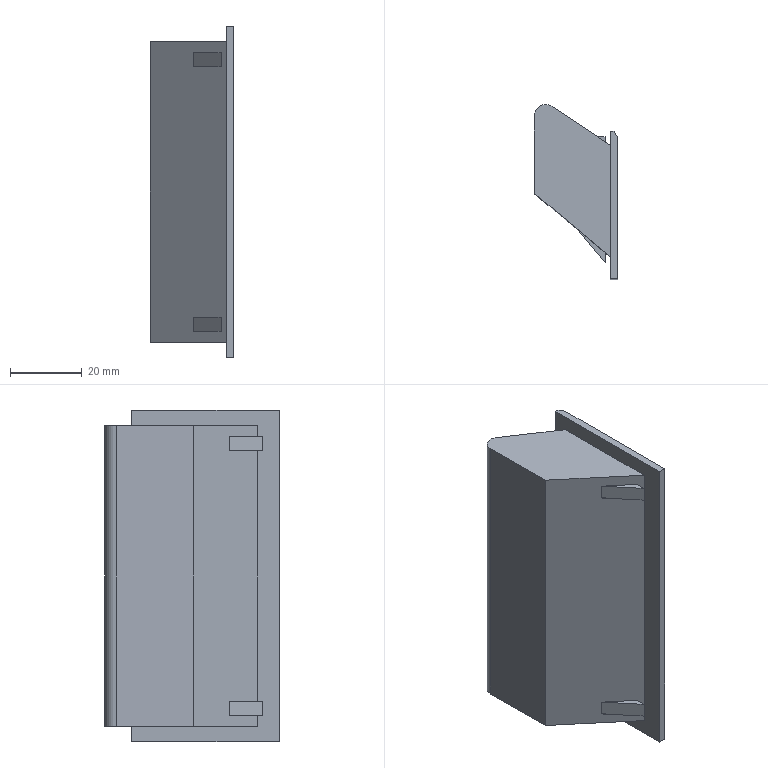Part | SolidWorks | features BaseBody 1 | 1 solid | 54 faces | box 23.155 x 48.5 x 92 mm | volume 9910 mm3 | plane 52 | cylinder 2 | commonest cylinder face diameters 4 x1 6.309 x1
STEP:
#1=CARTESIAN_POINT('',(-22.,24.19,40.75));
#2=VERTEX_POINT('',#1);
#3=CARTESIAN_POINT('',(0.,5.73,40.75));
#4=VERTEX_POINT('',#3);
#5=CARTESIAN_POINT('',(-22.,24.19,40.75));
#6=DIRECTION('',(0.766,-0.6428,0.));
#7=VECTOR('',#6,1000.);
#8=LINE('',#5,#7);
#9=EDGE_CURVE('',#2,#4,#8,.T.);
#10=ORIENTED_EDGE('',*,*,#9,.T.);
#11=CARTESIAN_POINT('',(0.,5.73,-40.75));
#12=VERTEX_POINT('',#11);
#13=CARTESIAN_POINT('',(0.,5.73,40.75));
#14=DIRECTION('',(0.,0.,-1.));
#15=VECTOR('',#14,1000.);
#16=LINE('',#13,#15);
#17=EDGE_CURVE('',#4,#12,#16,.T.);
#18=ORIENTED_EDGE('',*,*,#17,.T.);
#19=CARTESIAN_POINT('',(-22.,24.19,-40.75));
#20=VERTEX_POINT('',#19);
#21=CARTESIAN_POINT('',(-22.,24.19,-40.75));
#22=DIRECTION('',(-0.766,0.6428,0.));
#23=VECTOR('',#22,1000.);
#24=LINE('',#21,#23);
#25=EDGE_CURVE('',#12,#20,#24,.T.);
#26=ORIENTED_EDGE('',*,*,#25,.T.);
#27=CARTESIAN_POINT('',(-22.,24.19,40.75));
#28=DIRECTION('',(0.,0.,1.));
#29=VECTOR('',#28,1000.);
#30=LINE('',#27,#29);
#31=EDGE_CURVE('',#20,#2,#30,.T.);
#32=ORIENTED_EDGE('',*,*,#31,.T.);
#33=EDGE_LOOP('',(#10,#18,#26,#32));
#34=FACE_OUTER_BOUND('',#33,.T.);
#35=CARTESIAN_POINT('',(-22.,24.19,40.75));
#36=DIRECTION('',(0.6428,0.766,0.));
#37=DIRECTION('',(-0.766,0.6428,0.));
#38=AXIS2_PLACEMENT_3D('',#35,#36,#37);
#39=PLANE('',#38);
#40=ADVANCED_FACE('',(#34),#39,.T.);
#41=CARTESIAN_POINT('',(0.,39.268,46.));
#42=VERTEX_POINT('',#41);
#43=CARTESIAN_POINT('',(0.,39.268,-46.));
#44=VERTEX_POINT('',#43);
#45=CARTESIAN_POINT('',(0.,39.268,46.));
#46=DIRECTION('',(0.,0.,-1.));
#47=VECTOR('',#46,1000.);
#48=LINE('',#45,#47);
#49=EDGE_CURVE('',#42,#44,#48,.T.);
#50=ORIENTED_EDGE('',*,*,#49,.F.);
#51=CARTESIAN_POINT('',(0.,0.,46.));
#52=VERTEX_POINT('',#51);
#53=CARTESIAN_POINT('',(0.,0.,46.));
#54=DIRECTION('',(0.,1.,0.));
#55=VECTOR('',#54,1000.);
#56=LINE('',#53,#55);
#57=EDGE_CURVE('',#52,#42,#56,.T.);
#58=ORIENTED_EDGE('',*,*,#57,.F.);
#59=CARTESIAN_POINT('',(0.,0.,-46.));
#60=VERTEX_POINT('',#59);
#61=CARTESIAN_POINT('',(0.,0.,46.));
#62=DIRECTION('',(0.,0.,1.));
#63=VECTOR('',#62,1000.);
#64=LINE('',#61,#63);
#65=EDGE_CURVE('',#60,#52,#64,.T.);
#66=ORIENTED_EDGE('',*,*,#65,.F.);
#67=CARTESIAN_POINT('',(0.,0.,-46.));
#68=DIRECTION('',(0.,-1.,0.));
#69=VECTOR('',#68,1000.);
#70=LINE('',#67,#69);
#71=EDGE_CURVE('',#44,#60,#70,.T.);
#72=ORIENTED_EDGE('',*,*,#71,.F.);
#73=EDGE_LOOP('',(#50,#58,#66,#72));
#74=FACE_OUTER_BOUND('',#73,.T.);
#75=CARTESIAN_POINT('',(0.,35.072,40.75));
#76=VERTEX_POINT('',#75);
#77=CARTESIAN_POINT('',(0.,0.,40.75));
#78=DIRECTION('',(0.,-1.,0.));
#79=VECTOR('',#78,1000.);
#80=LINE('',#77,#79);
#81=EDGE_CURVE('',#76,#4,#80,.T.);
#82=ORIENTED_EDGE('',*,*,#81,.F.);
#83=CARTESIAN_POINT('',(0.,35.072,-40.75));
#84=VERTEX_POINT('',#83);
#85=CARTESIAN_POINT('',(0.,35.072,46.));
#86=DIRECTION('',(0.,0.,1.));
#87=VECTOR('',#86,1000.);
#88=LINE('',#85,#87);
#89=EDGE_CURVE('',#84,#76,#88,.T.);
#90=ORIENTED_EDGE('',*,*,#89,.F.);
#91=CARTESIAN_POINT('',(0.,0.,-40.75));
#92=DIRECTION('',(0.,1.,0.));
#93=VECTOR('',#92,1000.);
#94=LINE('',#91,#93);
#95=EDGE_CURVE('',#12,#84,#94,.T.);
#96=ORIENTED_EDGE('',*,*,#95,.F.);
#97=ORIENTED_EDGE('',*,*,#17,.F.);
#98=EDGE_LOOP('',(#82,#90,#96,#97));
#99=FACE_BOUND('',#98,.T.);
#100=CARTESIAN_POINT('',(0.,0.,46.));
#101=DIRECTION('',(-1.,0.,0.));
#102=DIRECTION('',(0.,0.,1.));
#103=AXIS2_PLACEMENT_3D('',#100,#101,#102);
#104=PLANE('',#103);
#105=ADVANCED_FACE('',(#74,#99),#104,.F.);
#106=CARTESIAN_POINT('',(-18.919,47.184,40.75));
#107=VERTEX_POINT('',#106);
#108=CARTESIAN_POINT('',(-21.998,45.5,40.75));
#109=VERTEX_POINT('',#108);
#110=CARTESIAN_POINT('',(-19.998,45.5,40.75));
#111=DIRECTION('',(0.,0.,1.));
#112=DIRECTION('',(1.,0.,0.));
#113=AXIS2_PLACEMENT_3D('',#110,#111,#112);
#114=CIRCLE('',#113,2.);
#115=EDGE_CURVE('',#107,#109,#114,.T.);
#116=ORIENTED_EDGE('',*,*,#115,.F.);
#117=CARTESIAN_POINT('',(0.,35.072,40.75));
#118=DIRECTION('',(-0.8422,0.5392,0.));
#119=VECTOR('',#118,1000.);
#120=LINE('',#117,#119);
#121=EDGE_CURVE('',#76,#107,#120,.T.);
#122=ORIENTED_EDGE('',*,*,#121,.F.);
#123=ORIENTED_EDGE('',*,*,#81,.T.);
#124=ORIENTED_EDGE('',*,*,#9,.F.);
#125=CARTESIAN_POINT('',(-21.998,45.5,40.75));
#126=DIRECTION('',(-0.0001084,-1.,0.));
#127=VECTOR('',#126,1000.);
#128=LINE('',#125,#127);
#129=EDGE_CURVE('',#109,#2,#128,.T.);
#130=ORIENTED_EDGE('',*,*,#129,.F.);
#131=EDGE_LOOP('',(#116,#122,#123,#124,#130));
#132=FACE_OUTER_BOUND('',#131,.T.);
#133=CARTESIAN_POINT('',(-19.998,45.5,40.75));
#134=DIRECTION('',(0.,0.,1.));
#135=DIRECTION('',(1.,0.,0.));
#136=AXIS2_PLACEMENT_3D('',#133,#134,#135);
#137=PLANE('',#136);
#138=ADVANCED_FACE('',(#132),#137,.F.);
#139=ORIENTED_EDGE('',*,*,#129,.T.);
#140=ORIENTED_EDGE('',*,*,#31,.F.);
#141=CARTESIAN_POINT('',(-21.998,45.5,-40.75));
#142=VERTEX_POINT('',#141);
#143=CARTESIAN_POINT('',(-21.998,45.5,-40.75));
#144=DIRECTION('',(0.0001084,1.,0.));
#145=VECTOR('',#144,1000.);
#146=LINE('',#143,#145);
#147=EDGE_CURVE('',#20,#142,#146,.T.);
#148=ORIENTED_EDGE('',*,*,#147,.T.);
#149=CARTESIAN_POINT('',(-21.998,45.5,40.75));
#150=DIRECTION('',(0.,0.,1.));
#151=VECTOR('',#150,1000.);
#152=LINE('',#149,#151);
#153=EDGE_CURVE('',#142,#109,#152,.T.);
#154=ORIENTED_EDGE('',*,*,#153,.T.);
#155=EDGE_LOOP('',(#139,#140,#148,#154));
#156=FACE_OUTER_BOUND('',#155,.T.);
#157=CARTESIAN_POINT('',(-21.998,45.5,40.75));
#158=DIRECTION('',(1.,-0.0001084,0.));
#159=DIRECTION('',(0.0001084,1.,0.));
#160=AXIS2_PLACEMENT_3D('',#157,#158,#159);
#161=PLANE('',#160);
#162=ADVANCED_FACE('',(#156),#161,.T.);
#163=CARTESIAN_POINT('',(-18.919,47.184,-40.75));
#164=VERTEX_POINT('',#163);
#165=CARTESIAN_POINT('',(0.,35.072,-40.75));
#166=DIRECTION('',(-0.8422,0.5392,0.));
#167=VECTOR('',#166,1000.);
#168=LINE('',#165,#167);
#169=EDGE_CURVE('',#84,#164,#168,.T.);
#170=ORIENTED_EDGE('',*,*,#169,.T.);
#171=CARTESIAN_POINT('',(-19.998,45.5,-40.75));
#172=DIRECTION('',(0.,0.,1.));
#173=DIRECTION('',(1.,0.,0.));
#174=AXIS2_PLACEMENT_3D('',#171,#172,#173);
#175=CIRCLE('',#174,2.);
#176=EDGE_CURVE('',#164,#142,#175,.T.);
#177=ORIENTED_EDGE('',*,*,#176,.T.);
#178=ORIENTED_EDGE('',*,*,#147,.F.);
#179=ORIENTED_EDGE('',*,*,#25,.F.);
#180=ORIENTED_EDGE('',*,*,#95,.T.);
#181=EDGE_LOOP('',(#170,#177,#178,#179,#180));
#182=FACE_OUTER_BOUND('',#181,.T.);
#183=CARTESIAN_POINT('',(-19.998,45.5,-40.75));
#184=DIRECTION('',(0.,0.,1.));
#185=DIRECTION('',(1.,0.,0.));
#186=AXIS2_PLACEMENT_3D('',#183,#184,#185);
#187=PLANE('',#186);
#188=ADVANCED_FACE('',(#182),#187,.T.);
#189=CARTESIAN_POINT('',(-1.,41.,-46.));
#190=VERTEX_POINT('',#189);
#191=CARTESIAN_POINT('',(0.,39.268,-46.));
#192=DIRECTION('',(-0.5,0.866,0.));
#193=VECTOR('',#192,1000.);
#194=LINE('',#191,#193);
#195=EDGE_CURVE('',#44,#190,#194,.T.);
#196=ORIENTED_EDGE('',*,*,#195,.F.);
#197=ORIENTED_EDGE('',*,*,#71,.T.);
#198=CARTESIAN_POINT('',(-2.,0.,-46.));
#199=VERTEX_POINT('',#198);
#200=CARTESIAN_POINT('',(0.,0.,-46.));
#201=DIRECTION('',(1.,0.,0.));
#202=VECTOR('',#201,1000.);
#203=LINE('',#200,#202);
#204=EDGE_CURVE('',#199,#60,#203,.T.);
#205=ORIENTED_EDGE('',*,*,#204,.F.);
#206=CARTESIAN_POINT('',(-2.,41.,-46.));
#207=VERTEX_POINT('',#206);
#208=CARTESIAN_POINT('',(-2.,0.,-46.));
#209=DIRECTION('',(0.,-1.,0.));
#210=VECTOR('',#209,1000.);
#211=LINE('',#208,#210);
#212=EDGE_CURVE('',#207,#199,#211,.T.);
#213=ORIENTED_EDGE('',*,*,#212,.F.);
#214=CARTESIAN_POINT('',(-1.,41.,-46.));
#215=DIRECTION('',(1.,0.,0.));
#216=VECTOR('',#215,1000.);
#217=LINE('',#214,#216);
#218=EDGE_CURVE('',#207,#190,#217,.T.);
#219=ORIENTED_EDGE('',*,*,#218,.T.);
#220=EDGE_LOOP('',(#196,#197,#205,#213,#219));
#221=FACE_OUTER_BOUND('',#220,.T.);
#222=CARTESIAN_POINT('',(0.,0.,-46.));
#223=DIRECTION('',(0.,0.,1.));
#224=DIRECTION('',(1.,0.,0.));
#225=AXIS2_PLACEMENT_3D('',#222,#223,#224);
#226=PLANE('',#225);
#227=ADVANCED_FACE('',(#221),#226,.F.);
#228=CARTESIAN_POINT('',(-1.,41.,46.));
#229=VERTEX_POINT('',#228);
#230=CARTESIAN_POINT('',(-1.,41.,46.));
#231=DIRECTION('',(0.,0.,-1.));
#232=VECTOR('',#231,1000.);
#233=LINE('',#230,#232);
#234=EDGE_CURVE('',#229,#190,#233,.T.);
#235=ORIENTED_EDGE('',*,*,#234,.F.);
#236=CARTESIAN_POINT('',(0.,39.268,46.));
#237=DIRECTION('',(-0.5,0.866,0.));
#238=VECTOR('',#237,1000.);
#239=LINE('',#236,#238);
#240=EDGE_CURVE('',#42,#229,#239,.T.);
#241=ORIENTED_EDGE('',*,*,#240,.F.);
#242=ORIENTED_EDGE('',*,*,#49,.T.);
#243=ORIENTED_EDGE('',*,*,#195,.T.);
#244=EDGE_LOOP('',(#235,#241,#242,#243));
#245=FACE_OUTER_BOUND('',#244,.T.);
#246=CARTESIAN_POINT('',(0.,39.268,46.));
#247=DIRECTION('',(-0.866,-0.5,0.));
#248=DIRECTION('',(0.5,-0.866,0.));
#249=AXIS2_PLACEMENT_3D('',#246,#247,#248);
#250=PLANE('',#249);
#251=ADVANCED_FACE('',(#245),#250,.F.);
#252=ORIENTED_EDGE('',*,*,#57,.T.);
#253=ORIENTED_EDGE('',*,*,#240,.T.);
#254=CARTESIAN_POINT('',(-2.,41.,46.));
#255=VERTEX_POINT('',#254);
#256=CARTESIAN_POINT('',(0.,41.,46.));
#257=DIRECTION('',(-1.,0.,0.));
#258=VECTOR('',#257,1000.);
#259=LINE('',#256,#258);
#260=EDGE_CURVE('',#229,#255,#259,.T.);
#261=ORIENTED_EDGE('',*,*,#260,.T.);
#262=CARTESIAN_POINT('',(-2.,0.,46.));
#263=VERTEX_POINT('',#262);
#264=CARTESIAN_POINT('',(-2.,0.,46.));
#265=DIRECTION('',(0.,-1.,0.));
#266=VECTOR('',#265,1000.);
#267=LINE('',#264,#266);
#268=EDGE_CURVE('',#255,#263,#267,.T.);
#269=ORIENTED_EDGE('',*,*,#268,.T.);
#270=CARTESIAN_POINT('',(0.,0.,46.));
#271=DIRECTION('',(1.,0.,0.));
#272=VECTOR('',#271,1000.);
#273=LINE('',#270,#272);
#274=EDGE_CURVE('',#263,#52,#273,.T.);
#275=ORIENTED_EDGE('',*,*,#274,.T.);
#276=EDGE_LOOP('',(#252,#253,#261,#269,#275));
#277=FACE_OUTER_BOUND('',#276,.T.);
#278=CARTESIAN_POINT('',(0.,0.,46.));
#279=DIRECTION('',(0.,0.,1.));
#280=DIRECTION('',(1.,0.,0.));
#281=AXIS2_PLACEMENT_3D('',#278,#279,#280);
#282=PLANE('',#281);
#283=ADVANCED_FACE('',(#277),#282,.T.);
#284=ORIENTED_EDGE('',*,*,#65,.T.);
#285=ORIENTED_EDGE('',*,*,#274,.F.);
#286=CARTESIAN_POINT('',(-2.,0.,46.));
#287=DIRECTION('',(0.,0.,1.));
#288=VECTOR('',#287,1000.);
#289=LINE('',#286,#288);
#290=EDGE_CURVE('',#199,#263,#289,.T.);
#291=ORIENTED_EDGE('',*,*,#290,.F.);
#292=ORIENTED_EDGE('',*,*,#204,.T.);
#293=EDGE_LOOP('',(#284,#285,#291,#292));
#294=FACE_OUTER_BOUND('',#293,.T.);
#295=CARTESIAN_POINT('',(-2.,0.,46.));
#296=DIRECTION('',(0.,1.,0.));
#297=DIRECTION('',(0.,0.,1.));
#298=AXIS2_PLACEMENT_3D('',#295,#296,#297);
#299=PLANE('',#298);
#300=ADVANCED_FACE('',(#294),#299,.F.);
#301=CARTESIAN_POINT('',(-3.5,37.312,37.75));
#302=VERTEX_POINT('',#301);
#303=CARTESIAN_POINT('',(-3.5,37.312,35.75));
#304=VERTEX_POINT('',#303);
#305=CARTESIAN_POINT('',(-3.5,37.312,40.75));
#306=DIRECTION('',(0.,0.,-1.));
#307=VECTOR('',#306,1000.);
#308=LINE('',#305,#307);
#309=EDGE_CURVE('',#302,#304,#308,.T.);
#310=ORIENTED_EDGE('',*,*,#309,.T.);
#311=CARTESIAN_POINT('',(-6.917,39.5,35.75));
#312=VERTEX_POINT('',#311);
#313=CARTESIAN_POINT('',(0.,35.072,35.75));
#314=DIRECTION('',(-0.8422,0.5392,0.));
#315=VECTOR('',#314,1000.);
#316=LINE('',#313,#315);
#317=EDGE_CURVE('',#304,#312,#316,.T.);
#318=ORIENTED_EDGE('',*,*,#317,.T.);
#319=CARTESIAN_POINT('',(-6.917,39.5,37.75));
#320=VERTEX_POINT('',#319);
#321=CARTESIAN_POINT('',(-6.917,39.5,40.75));
#322=DIRECTION('',(0.,0.,1.));
#323=VECTOR('',#322,1000.);
#324=LINE('',#321,#323);
#325=EDGE_CURVE('',#312,#320,#324,.T.);
#326=ORIENTED_EDGE('',*,*,#325,.T.);
#327=CARTESIAN_POINT('',(0.,35.072,37.75));
#328=DIRECTION('',(0.8422,-0.5392,0.));
#329=VECTOR('',#328,1000.);
#330=LINE('',#327,#329);
#331=EDGE_CURVE('',#320,#302,#330,.T.);
#332=ORIENTED_EDGE('',*,*,#331,.T.);
#333=EDGE_LOOP('',(#310,#318,#326,#332));
#334=FACE_BOUND('',#333,.T.);
#335=CARTESIAN_POINT('',(-3.5,37.312,-35.75));
#336=VERTEX_POINT('',#335);
#337=CARTESIAN_POINT('',(-3.5,37.312,-37.75));
#338=VERTEX_POINT('',#337);
#339=CARTESIAN_POINT('',(-3.5,37.312,40.75));
#340=DIRECTION('',(0.,0.,-1.));
#341=VECTOR('',#340,1000.);
#342=LINE('',#339,#341);
#343=EDGE_CURVE('',#336,#338,#342,.T.);
#344=ORIENTED_EDGE('',*,*,#343,.T.);
#345=CARTESIAN_POINT('',(-6.917,39.5,-37.75));
#346=VERTEX_POINT('',#345);
#347=CARTESIAN_POINT('',(0.,35.072,-37.75));
#348=DIRECTION('',(-0.8422,0.5392,0.));
#349=VECTOR('',#348,1000.);
#350=LINE('',#347,#349);
#351=EDGE_CURVE('',#338,#346,#350,.T.);
#352=ORIENTED_EDGE('',*,*,#351,.T.);
#353=CARTESIAN_POINT('',(-6.917,39.5,-35.75));
#354=VERTEX_POINT('',#353);
#355=CARTESIAN_POINT('',(-6.917,39.5,40.75));
#356=DIRECTION('',(0.,0.,1.));
#357=VECTOR('',#356,1000.);
#358=LINE('',#355,#357);
#359=EDGE_CURVE('',#346,#354,#358,.T.);
#360=ORIENTED_EDGE('',*,*,#359,.T.);
#361=CARTESIAN_POINT('',(0.,35.072,-35.75));
#362=DIRECTION('',(0.8422,-0.5392,0.));
#363=VECTOR('',#362,1000.);
#364=LINE('',#361,#363);
#365=EDGE_CURVE('',#354,#336,#364,.T.);
#366=ORIENTED_EDGE('',*,*,#365,.T.);
#367=EDGE_LOOP('',(#344,#352,#360,#366));
#368=FACE_BOUND('',#367,.T.);
#369=CARTESIAN_POINT('',(-3.5,37.312,1.));
#370=VERTEX_POINT('',#369);
#371=CARTESIAN_POINT('',(-3.5,37.312,-1.));
#372=VERTEX_POINT('',#371);
#373=CARTESIAN_POINT('',(-3.5,37.312,40.75));
#374=DIRECTION('',(0.,0.,-1.));
#375=VECTOR('',#374,1000.);
#376=LINE('',#373,#375);
#377=EDGE_CURVE('',#370,#372,#376,.T.);
#378=ORIENTED_EDGE('',*,*,#377,.T.);
#379=CARTESIAN_POINT('',(-6.917,39.5,-1.));
#380=VERTEX_POINT('',#379);
#381=CARTESIAN_POINT('',(0.,35.072,-1.));
#382=DIRECTION('',(-0.8422,0.5392,0.));
#383=VECTOR('',#382,1000.);
#384=LINE('',#381,#383);
#385=EDGE_CURVE('',#372,#380,#384,.T.);
#386=ORIENTED_EDGE('',*,*,#385,.T.);
#387=CARTESIAN_POINT('',(-6.917,39.5,1.));
#388=VERTEX_POINT('',#387);
#389=CARTESIAN_POINT('',(-6.917,39.5,40.75));
#390=DIRECTION('',(0.,0.,1.));
#391=VECTOR('',#390,1000.);
#392=LINE('',#389,#391);
#393=EDGE_CURVE('',#380,#388,#392,.T.);
#394=ORIENTED_EDGE('',*,*,#393,.T.);
#395=CARTESIAN_POINT('',(0.,35.072,1.));
#396=DIRECTION('',(0.8422,-0.5392,0.));
#397=VECTOR('',#396,1000.);
#398=LINE('',#395,#397);
#399=EDGE_CURVE('',#388,#370,#398,.T.);
#400=ORIENTED_EDGE('',*,*,#399,.T.);
#401=EDGE_LOOP('',(#378,#386,#394,#400));
#402=FACE_BOUND('',#401,.T.);
#403=ORIENTED_EDGE('',*,*,#121,.T.);
#404=CARTESIAN_POINT('',(-18.919,47.184,40.75));
#405=DIRECTION('',(0.,0.,-1.));
#406=VECTOR('',#405,1000.);
#407=LINE('',#404,#406);
#408=EDGE_CURVE('',#107,#164,#407,.T.);
#409=ORIENTED_EDGE('',*,*,#408,.T.);
#410=ORIENTED_EDGE('',*,*,#169,.F.);
#411=ORIENTED_EDGE('',*,*,#89,.T.);
#412=EDGE_LOOP('',(#403,#409,#410,#411));
#413=FACE_OUTER_BOUND('',#412,.T.);
#414=CARTESIAN_POINT('',(0.,35.072,40.75));
#415=DIRECTION('',(-0.5392,-0.8422,0.));
#416=DIRECTION('',(0.8422,-0.5392,0.));
#417=AXIS2_PLACEMENT_3D('',#414,#415,#416);
#418=PLANE('',#417);
#419=ADVANCED_FACE('',(#334,#368,#402,#413),#418,.T.);
#420=ORIENTED_EDGE('',*,*,#408,.F.);
#421=ORIENTED_EDGE('',*,*,#115,.T.);
#422=ORIENTED_EDGE('',*,*,#153,.F.);
#423=ORIENTED_EDGE('',*,*,#176,.F.);
#424=EDGE_LOOP('',(#420,#421,#422,#423));
#425=FACE_OUTER_BOUND('',#424,.T.);
#426=CARTESIAN_POINT('',(-19.998,45.5,40.75));
#427=DIRECTION('',(0.,0.,1.));
#428=DIRECTION('',(1.,0.,0.));
#429=AXIS2_PLACEMENT_3D('',#426,#427,#428);
#430=CYLINDRICAL_SURFACE('',#429,2.);
#431=ADVANCED_FACE('',(#425),#430,.F.);
#432=ORIENTED_EDGE('',*,*,#290,.T.);
#433=ORIENTED_EDGE('',*,*,#268,.F.);
#434=CARTESIAN_POINT('',(-2.,41.,46.));
#435=DIRECTION('',(0.,0.,1.));
#436=VECTOR('',#435,1000.);
#437=LINE('',#434,#436);
#438=EDGE_CURVE('',#207,#255,#437,.T.);
#439=ORIENTED_EDGE('',*,*,#438,.F.);
#440=ORIENTED_EDGE('',*,*,#212,.T.);
#441=EDGE_LOOP('',(#432,#433,#439,#440));
#442=FACE_OUTER_BOUND('',#441,.T.);
#443=CARTESIAN_POINT('',(-2.,37.108,-41.75));
#444=VERTEX_POINT('',#443);
#445=CARTESIAN_POINT('',(-2.,6.103,-41.75));
#446=VERTEX_POINT('',#445);
#447=CARTESIAN_POINT('',(-2.,41.,-41.75));
#448=DIRECTION('',(0.,-1.,0.));
#449=VECTOR('',#448,1000.);
#450=LINE('',#447,#449);
#451=EDGE_CURVE('',#444,#446,#450,.T.);
#452=ORIENTED_EDGE('',*,*,#451,.F.);
#453=CARTESIAN_POINT('',(-2.,37.108,41.75));
#454=VERTEX_POINT('',#453);
#455=CARTESIAN_POINT('',(-2.,37.108,46.));
#456=DIRECTION('',(0.,0.,-1.));
#457=VECTOR('',#456,1000.);
#458=LINE('',#455,#457);
#459=EDGE_CURVE('',#454,#444,#458,.T.);
#460=ORIENTED_EDGE('',*,*,#459,.F.);
#461=CARTESIAN_POINT('',(-2.,6.103,41.75));
#462=VERTEX_POINT('',#461);
#463=CARTESIAN_POINT('',(-2.,41.,41.75));
#464=DIRECTION('',(0.,1.,0.));
#465=VECTOR('',#464,1000.);
#466=LINE('',#463,#465);
#467=EDGE_CURVE('',#462,#454,#466,.T.);
#468=ORIENTED_EDGE('',*,*,#467,.F.);
#469=CARTESIAN_POINT('',(-2.,6.103,46.));
#470=DIRECTION('',(0.,0.,1.));
#471=VECTOR('',#470,1000.);
#472=LINE('',#469,#471);
#473=EDGE_CURVE('',#446,#462,#472,.T.);
#474=ORIENTED_EDGE('',*,*,#473,.F.);
#475=EDGE_LOOP('',(#452,#460,#468,#474));
#476=FACE_BOUND('',#475,.T.);
#477=CARTESIAN_POINT('',(-2.,41.,46.));
#478=DIRECTION('',(1.,0.,0.));
#479=DIRECTION('',(0.,0.,-1.));
#480=AXIS2_PLACEMENT_3D('',#477,#478,#479);
#481=PLANE('',#480);
#482=ADVANCED_FACE('',(#442,#476),#481,.F.);
#483=ORIENTED_EDGE('',*,*,#438,.T.);
#484=ORIENTED_EDGE('',*,*,#260,.F.);
#485=ORIENTED_EDGE('',*,*,#234,.T.);
#486=ORIENTED_EDGE('',*,*,#218,.F.);
#487=EDGE_LOOP('',(#483,#484,#485,#486));
#488=FACE_OUTER_BOUND('',#487,.T.);
#489=CARTESIAN_POINT('',(-1.,41.,46.));
#490=DIRECTION('',(0.,-1.,0.));
#491=DIRECTION('',(0.,0.,-1.));
#492=AXIS2_PLACEMENT_3D('',#489,#490,#491);
#493=PLANE('',#492);
#494=ADVANCED_FACE('',(#488),#493,.F.);
#495=CARTESIAN_POINT('',(-3.5,37.304,35.75));
#496=VERTEX_POINT('',#495);
#497=CARTESIAN_POINT('',(-3.5,0.,35.75));
#498=DIRECTION('',(0.,-1.,0.));
#499=VECTOR('',#498,1000.);
#500=LINE('',#497,#499);
#501=EDGE_CURVE('',#304,#496,#500,.T.);
#502=ORIENTED_EDGE('',*,*,#501,.T.);
#503=CARTESIAN_POINT('',(-8.21,39.5,35.75));
#504=VERTEX_POINT('',#503);
#505=CARTESIAN_POINT('',(-3.5,37.304,35.75));
#506=DIRECTION('',(-0.9063,0.4226,0.));
#507=VECTOR('',#506,1000.);
#508=LINE('',#505,#507);
#509=EDGE_CURVE('',#496,#504,#508,.T.);
#510=ORIENTED_EDGE('',*,*,#509,.T.);
#511=CARTESIAN_POINT('',(0.,39.5,35.75));
#512=DIRECTION('',(1.,0.,0.));
#513=VECTOR('',#512,1000.);
#514=LINE('',#511,#513);
#515=EDGE_CURVE('',#504,#312,#514,.T.);
#516=ORIENTED_EDGE('',*,*,#515,.T.);
#517=ORIENTED_EDGE('',*,*,#317,.F.);
#518=EDGE_LOOP('',(#502,#510,#516,#517));
#519=FACE_OUTER_BOUND('',#518,.T.);
#520=CARTESIAN_POINT('',(0.,0.,35.75));
#521=DIRECTION('',(0.,0.,-1.));
#522=DIRECTION('',(-1.,0.,0.));
#523=AXIS2_PLACEMENT_3D('',#520,#521,#522);
#524=PLANE('',#523);
#525=ADVANCED_FACE('',(#519),#524,.T.);
#526=CARTESIAN_POINT('',(-3.5,37.304,37.75));
#527=VERTEX_POINT('',#526);
#528=CARTESIAN_POINT('',(-3.5,37.304,37.75));
#529=DIRECTION('',(0.,1.,0.));
#530=VECTOR('',#529,1000.);
#531=LINE('',#528,#530);
#532=EDGE_CURVE('',#527,#302,#531,.T.);
#533=ORIENTED_EDGE('',*,*,#532,.F.);
#534=CARTESIAN_POINT('',(-3.5,37.304,37.75));
#535=DIRECTION('',(0.,0.,1.));
#536=VECTOR('',#535,1000.);
#537=LINE('',#534,#536);
#538=EDGE_CURVE('',#496,#527,#537,.T.);
#539=ORIENTED_EDGE('',*,*,#538,.F.);
#540=ORIENTED_EDGE('',*,*,#501,.F.);
#541=ORIENTED_EDGE('',*,*,#309,.F.);
#542=EDGE_LOOP('',(#533,#539,#540,#541));
#543=FACE_OUTER_BOUND('',#542,.T.);
#544=CARTESIAN_POINT('',(-3.5,37.304,37.75));
#545=DIRECTION('',(-1.,0.,0.));
#546=DIRECTION('',(0.,0.,1.));
#547=AXIS2_PLACEMENT_3D('',#544,#545,#546);
#548=PLANE('',#547);
#549=ADVANCED_FACE('',(#543),#548,.F.);
#550=CARTESIAN_POINT('',(-8.21,39.5,37.75));
#551=VERTEX_POINT('',#550);
#552=CARTESIAN_POINT('',(0.,39.5,37.75));
#553=DIRECTION('',(1.,0.,0.));
#554=VECTOR('',#553,1000.);
#555=LINE('',#552,#554);
#556=EDGE_CURVE('',#551,#320,#555,.T.);
#557=ORIENTED_EDGE('',*,*,#556,.F.);
#558=CARTESIAN_POINT('',(-3.5,37.304,37.75));
#559=DIRECTION('',(-0.9063,0.4226,0.));
#560=VECTOR('',#559,1000.);
#561=LINE('',#558,#560);
#562=EDGE_CURVE('',#527,#551,#561,.T.);
#563=ORIENTED_EDGE('',*,*,#562,.F.);
#564=ORIENTED_EDGE('',*,*,#532,.T.);
#565=ORIENTED_EDGE('',*,*,#331,.F.);
#566=EDGE_LOOP('',(#557,#563,#564,#565));
#567=FACE_OUTER_BOUND('',#566,.T.);
#568=CARTESIAN_POINT('',(0.,0.,37.75));
#569=DIRECTION('',(0.,0.,-1.));
#570=DIRECTION('',(-1.,0.,0.));
#571=AXIS2_PLACEMENT_3D('',#568,#569,#570);
#572=PLANE('',#571);
#573=ADVANCED_FACE('',(#567),#572,.F.);
#574=ORIENTED_EDGE('',*,*,#515,.F.);
#575=CARTESIAN_POINT('',(-8.21,39.5,37.75));
#576=DIRECTION('',(0.,0.,-1.));
#577=VECTOR('',#576,1000.);
#578=LINE('',#575,#577);
#579=EDGE_CURVE('',#551,#504,#578,.T.);
#580=ORIENTED_EDGE('',*,*,#579,.F.);
#581=ORIENTED_EDGE('',*,*,#556,.T.);
#582=ORIENTED_EDGE('',*,*,#325,.F.);
#583=EDGE_LOOP('',(#574,#580,#581,#582));
#584=FACE_OUTER_BOUND('',#583,.T.);
#585=CARTESIAN_POINT('',(-3.5,39.5,37.75));
#586=DIRECTION('',(0.,-1.,0.));
#587=DIRECTION('',(0.,0.,-1.));
#588=AXIS2_PLACEMENT_3D('',#585,#586,#587);
#589=PLANE('',#588);
#590=ADVANCED_FACE('',(#584),#589,.F.);
#591=CARTESIAN_POINT('',(-3.5,37.304,-37.75));
#592=VERTEX_POINT('',#591);
#593=CARTESIAN_POINT('',(-3.5,0.,-37.75));
#594=DIRECTION('',(0.,-1.,0.));
#595=VECTOR('',#594,1000.);
#596=LINE('',#593,#595);
#597=EDGE_CURVE('',#338,#592,#596,.T.);
#598=ORIENTED_EDGE('',*,*,#597,.T.);
#599=CARTESIAN_POINT('',(-8.21,39.5,-37.75));
#600=VERTEX_POINT('',#599);
#601=CARTESIAN_POINT('',(-3.5,37.304,-37.75));
#602=DIRECTION('',(-0.9063,0.4226,0.));
#603=VECTOR('',#602,1000.);
#604=LINE('',#601,#603);
#605=EDGE_CURVE('',#592,#600,#604,.T.);
#606=ORIENTED_EDGE('',*,*,#605,.T.);
#607=CARTESIAN_POINT('',(0.,39.5,-37.75));
#608=DIRECTION('',(1.,0.,0.));
#609=VECTOR('',#608,1000.);
#610=LINE('',#607,#609);
#611=EDGE_CURVE('',#600,#346,#610,.T.);
#612=ORIENTED_EDGE('',*,*,#611,.T.);
#613=ORIENTED_EDGE('',*,*,#351,.F.);
#614=EDGE_LOOP('',(#598,#606,#612,#613));
#615=FACE_OUTER_BOUND('',#614,.T.);
#616=CARTESIAN_POINT('',(0.,0.,-37.75));
#617=DIRECTION('',(0.,0.,-1.));
#618=DIRECTION('',(-1.,0.,0.));
#619=AXIS2_PLACEMENT_3D('',#616,#617,#618);
#620=PLANE('',#619);
#621=ADVANCED_FACE('',(#615),#620,.T.);
#622=CARTESIAN_POINT('',(-3.5,37.304,-35.75));
#623=VERTEX_POINT('',#622);
#624=CARTESIAN_POINT('',(-3.5,37.304,-35.75));
#625=DIRECTION('',(0.,1.,0.));
#626=VECTOR('',#625,1000.);
#627=LINE('',#624,#626);
#628=EDGE_CURVE('',#623,#336,#627,.T.);
#629=ORIENTED_EDGE('',*,*,#628,.F.);
#630=CARTESIAN_POINT('',(-3.5,37.304,-35.75));
#631=DIRECTION('',(0.,0.,1.));
#632=VECTOR('',#631,1000.);
#633=LINE('',#630,#632);
#634=EDGE_CURVE('',#592,#623,#633,.T.);
#635=ORIENTED_EDGE('',*,*,#634,.F.);
#636=ORIENTED_EDGE('',*,*,#597,.F.);
#637=ORIENTED_EDGE('',*,*,#343,.F.);
#638=EDGE_LOOP('',(#629,#635,#636,#637));
#639=FACE_OUTER_BOUND('',#638,.T.);
#640=CARTESIAN_POINT('',(-3.5,37.304,-35.75));
#641=DIRECTION('',(-1.,0.,0.));
#642=DIRECTION('',(0.,0.,1.));
#643=AXIS2_PLACEMENT_3D('',#640,#641,#642);
#644=PLANE('',#643);
#645=ADVANCED_FACE('',(#639),#644,.F.);
#646=CARTESIAN_POINT('',(-8.21,39.5,-35.75));
#647=VERTEX_POINT('',#646);
#648=CARTESIAN_POINT('',(0.,39.5,-35.75));
#649=DIRECTION('',(1.,0.,0.));
#650=VECTOR('',#649,1000.);
#651=LINE('',#648,#650);
#652=EDGE_CURVE('',#647,#354,#651,.T.);
#653=ORIENTED_EDGE('',*,*,#652,.F.);
#654=CARTESIAN_POINT('',(-3.5,37.304,-35.75));
#655=DIRECTION('',(-0.9063,0.4226,0.));
#656=VECTOR('',#655,1000.);
#657=LINE('',#654,#656);
#658=EDGE_CURVE('',#623,#647,#657,.T.);
#659=ORIENTED_EDGE('',*,*,#658,.F.);
#660=ORIENTED_EDGE('',*,*,#628,.T.);
#661=ORIENTED_EDGE('',*,*,#365,.F.);
#662=EDGE_LOOP('',(#653,#659,#660,#661));
#663=FACE_OUTER_BOUND('',#662,.T.);
#664=CARTESIAN_POINT('',(0.,0.,-35.75));
#665=DIRECTION('',(0.,0.,-1.));
#666=DIRECTION('',(-1.,0.,0.));
#667=AXIS2_PLACEMENT_3D('',#664,#665,#666);
#668=PLANE('',#667);
#669=ADVANCED_FACE('',(#663),#668,.F.);
#670=ORIENTED_EDGE('',*,*,#611,.F.);
#671=CARTESIAN_POINT('',(-8.21,39.5,-35.75));
#672=DIRECTION('',(0.,0.,-1.));
#673=VECTOR('',#672,1000.);
#674=LINE('',#671,#673);
#675=EDGE_CURVE('',#647,#600,#674,.T.);
#676=ORIENTED_EDGE('',*,*,#675,.F.);
#677=ORIENTED_EDGE('',*,*,#652,.T.);
#678=ORIENTED_EDGE('',*,*,#359,.F.);
#679=EDGE_LOOP('',(#670,#676,#677,#678));
#680=FACE_OUTER_BOUND('',#679,.T.);
#681=CARTESIAN_POINT('',(-3.5,39.5,-35.75));
#682=DIRECTION('',(0.,-1.,0.));
#683=DIRECTION('',(0.,0.,-1.));
#684=AXIS2_PLACEMENT_3D('',#681,#682,#683);
#685=PLANE('',#684);
#686=ADVANCED_FACE('',(#680),#685,.F.);
#687=CARTESIAN_POINT('',(-3.5,37.304,-1.));
#688=VERTEX_POINT('',#687);
#689=CARTESIAN_POINT('',(-3.5,0.,-1.));
#690=DIRECTION('',(0.,-1.,0.));
#691=VECTOR('',#690,1000.);
#692=LINE('',#689,#691);
#693=EDGE_CURVE('',#372,#688,#692,.T.);
#694=ORIENTED_EDGE('',*,*,#693,.T.);
#695=CARTESIAN_POINT('',(-8.21,39.5,-1.));
#696=VERTEX_POINT('',#695);
#697=CARTESIAN_POINT('',(-3.5,37.304,-1.));
#698=DIRECTION('',(-0.9063,0.4226,0.));
#699=VECTOR('',#698,1000.);
#700=LINE('',#697,#699);
#701=EDGE_CURVE('',#688,#696,#700,.T.);
#702=ORIENTED_EDGE('',*,*,#701,.T.);
#703=CARTESIAN_POINT('',(0.,39.5,-1.));
#704=DIRECTION('',(1.,0.,0.));
#705=VECTOR('',#704,1000.);
#706=LINE('',#703,#705);
#707=EDGE_CURVE('',#696,#380,#706,.T.);
#708=ORIENTED_EDGE('',*,*,#707,.T.);
#709=ORIENTED_EDGE('',*,*,#385,.F.);
#710=EDGE_LOOP('',(#694,#702,#708,#709));
#711=FACE_OUTER_BOUND('',#710,.T.);
#712=CARTESIAN_POINT('',(0.,0.,-1.));
#713=DIRECTION('',(0.,0.,-1.));
#714=DIRECTION('',(-1.,0.,0.));
#715=AXIS2_PLACEMENT_3D('',#712,#713,#714);
#716=PLANE('',#715);
#717=ADVANCED_FACE('',(#711),#716,.T.);
#718=CARTESIAN_POINT('',(-3.5,37.304,1.));
#719=VERTEX_POINT('',#718);
#720=CARTESIAN_POINT('',(-3.5,37.304,1.));
#721=DIRECTION('',(0.,1.,0.));
#722=VECTOR('',#721,1000.);
#723=LINE('',#720,#722);
#724=EDGE_CURVE('',#719,#370,#723,.T.);
#725=ORIENTED_EDGE('',*,*,#724,.F.);
#726=CARTESIAN_POINT('',(-3.5,37.304,1.));
#727=DIRECTION('',(0.,0.,1.));
#728=VECTOR('',#727,1000.);
#729=LINE('',#726,#728);
#730=EDGE_CURVE('',#688,#719,#729,.T.);
#731=ORIENTED_EDGE('',*,*,#730,.F.);
#732=ORIENTED_EDGE('',*,*,#693,.F.);
#733=ORIENTED_EDGE('',*,*,#377,.F.);
#734=EDGE_LOOP('',(#725,#731,#732,#733));
#735=FACE_OUTER_BOUND('',#734,.T.);
#736=CARTESIAN_POINT('',(-3.5,37.304,1.));
#737=DIRECTION('',(-1.,0.,0.));
#738=DIRECTION('',(0.,0.,1.));
#739=AXIS2_PLACEMENT_3D('',#736,#737,#738);
#740=PLANE('',#739);
#741=ADVANCED_FACE('',(#735),#740,.F.);
#742=CARTESIAN_POINT('',(-8.21,39.5,1.));
#743=VERTEX_POINT('',#742);
#744=CARTESIAN_POINT('',(0.,39.5,1.));
#745=DIRECTION('',(1.,0.,0.));
#746=VECTOR('',#745,1000.);
#747=LINE('',#744,#746);
#748=EDGE_CURVE('',#743,#388,#747,.T.);
#749=ORIENTED_EDGE('',*,*,#748,.F.);
#750=CARTESIAN_POINT('',(-3.5,37.304,1.));
#751=DIRECTION('',(-0.9063,0.4226,0.));
#752=VECTOR('',#751,1000.);
#753=LINE('',#750,#752);
#754=EDGE_CURVE('',#719,#743,#753,.T.);
#755=ORIENTED_EDGE('',*,*,#754,.F.);
#756=ORIENTED_EDGE('',*,*,#724,.T.);
#757=ORIENTED_EDGE('',*,*,#399,.F.);
#758=EDGE_LOOP('',(#749,#755,#756,#757));
#759=FACE_OUTER_BOUND('',#758,.T.);
#760=CARTESIAN_POINT('',(0.,0.,1.));
#761=DIRECTION('',(0.,0.,-1.));
#762=DIRECTION('',(-1.,0.,0.));
#763=AXIS2_PLACEMENT_3D('',#760,#761,#762);
#764=PLANE('',#763);
#765=ADVANCED_FACE('',(#759),#764,.F.);
#766=ORIENTED_EDGE('',*,*,#707,.F.);
#767=CARTESIAN_POINT('',(-8.21,39.5,1.));
#768=DIRECTION('',(0.,0.,-1.));
#769=VECTOR('',#768,1000.);
#770=LINE('',#767,#769);
#771=EDGE_CURVE('',#743,#696,#770,.T.);
#772=ORIENTED_EDGE('',*,*,#771,.F.);
#773=ORIENTED_EDGE('',*,*,#748,.T.);
#774=ORIENTED_EDGE('',*,*,#393,.F.);
#775=EDGE_LOOP('',(#766,#772,#773,#774));
#776=FACE_OUTER_BOUND('',#775,.T.);
#777=CARTESIAN_POINT('',(-3.5,39.5,1.));
#778=DIRECTION('',(0.,-1.,0.));
#779=DIRECTION('',(0.,0.,-1.));
#780=AXIS2_PLACEMENT_3D('',#777,#778,#779);
#781=PLANE('',#780);
#782=ADVANCED_FACE('',(#776),#781,.F.);
#783=CARTESIAN_POINT('',(-3.5,7.361,34.75));
#784=VERTEX_POINT('',#783);
#785=CARTESIAN_POINT('',(-3.5,7.361,38.75));
#786=VERTEX_POINT('',#785);
#787=CARTESIAN_POINT('',(-3.5,7.361,41.75));
#788=DIRECTION('',(0.,0.,1.));
#789=VECTOR('',#788,1000.);
#790=LINE('',#787,#789);
#791=EDGE_CURVE('',#784,#786,#790,.T.);
#792=ORIENTED_EDGE('',*,*,#791,.F.);
#793=CARTESIAN_POINT('',(-11.201,13.824,34.75));
#794=VERTEX_POINT('',#793);
#795=CARTESIAN_POINT('',(-23.,23.724,34.75));
#796=DIRECTION('',(0.766,-0.6428,0.));
#797=VECTOR('',#796,1000.);
#798=LINE('',#795,#797);
#799=EDGE_CURVE('',#794,#784,#798,.T.);
#800=ORIENTED_EDGE('',*,*,#799,.F.);
#801=CARTESIAN_POINT('',(-11.201,13.824,38.75));
#802=VERTEX_POINT('',#801);
#803=CARTESIAN_POINT('',(-11.201,13.824,41.75));
#804=DIRECTION('',(0.,0.,-1.));
#805=VECTOR('',#804,1000.);
#806=LINE('',#803,#805);
#807=EDGE_CURVE('',#802,#794,#806,.T.);
#808=ORIENTED_EDGE('',*,*,#807,.F.);
#809=CARTESIAN_POINT('',(-23.,23.724,38.75));
#810=DIRECTION('',(-0.766,0.6428,0.));
#811=VECTOR('',#810,1000.);
#812=LINE('',#809,#811);
#813=EDGE_CURVE('',#786,#802,#812,.T.);
#814=ORIENTED_EDGE('',*,*,#813,.F.);
#815=EDGE_LOOP('',(#792,#800,#808,#814));
#816=FACE_BOUND('',#815,.T.);
#817=ORIENTED_EDGE('',*,*,#473,.T.);
#818=CARTESIAN_POINT('',(-23.,23.724,41.75));
#819=VERTEX_POINT('',#818);
#820=CARTESIAN_POINT('',(-23.,23.724,41.75));
#821=DIRECTION('',(0.766,-0.6428,0.));
#822=VECTOR('',#821,1000.);
#823=LINE('',#820,#822);
#824=EDGE_CURVE('',#819,#462,#823,.T.);
#825=ORIENTED_EDGE('',*,*,#824,.F.);
#826=CARTESIAN_POINT('',(-23.,23.724,-41.75));
#827=VERTEX_POINT('',#826);
#828=CARTESIAN_POINT('',(-23.,23.724,41.75));
#829=DIRECTION('',(0.,0.,1.));
#830=VECTOR('',#829,1000.);
#831=LINE('',#828,#830);
#832=EDGE_CURVE('',#827,#819,#831,.T.);
#833=ORIENTED_EDGE('',*,*,#832,.F.);
#834=CARTESIAN_POINT('',(-23.,23.724,-41.75));
#835=DIRECTION('',(-0.766,0.6428,0.));
#836=VECTOR('',#835,1000.);
#837=LINE('',#834,#836);
#838=EDGE_CURVE('',#446,#827,#837,.T.);
#839=ORIENTED_EDGE('',*,*,#838,.F.);
#840=EDGE_LOOP('',(#817,#825,#833,#839));
#841=FACE_OUTER_BOUND('',#840,.T.);
#842=CARTESIAN_POINT('',(-3.5,7.361,-38.75));
#843=VERTEX_POINT('',#842);
#844=CARTESIAN_POINT('',(-3.5,7.361,-34.75));
#845=VERTEX_POINT('',#844);
#846=CARTESIAN_POINT('',(-3.5,7.361,41.75));
#847=DIRECTION('',(0.,0.,1.));
#848=VECTOR('',#847,1000.);
#849=LINE('',#846,#848);
#850=EDGE_CURVE('',#843,#845,#849,.T.);
#851=ORIENTED_EDGE('',*,*,#850,.F.);
#852=CARTESIAN_POINT('',(-11.201,13.824,-38.75));
#853=VERTEX_POINT('',#852);
#854=CARTESIAN_POINT('',(-23.,23.724,-38.75));
#855=DIRECTION('',(0.766,-0.6428,0.));
#856=VECTOR('',#855,1000.);
#857=LINE('',#854,#856);
#858=EDGE_CURVE('',#853,#843,#857,.T.);
#859=ORIENTED_EDGE('',*,*,#858,.F.);
#860=CARTESIAN_POINT('',(-11.201,13.824,-34.75));
#861=VERTEX_POINT('',#860);
#862=CARTESIAN_POINT('',(-11.201,13.824,41.75));
#863=DIRECTION('',(0.,0.,-1.));
#864=VECTOR('',#863,1000.);
#865=LINE('',#862,#864);
#866=EDGE_CURVE('',#861,#853,#865,.T.);
#867=ORIENTED_EDGE('',*,*,#866,.F.);
#868=CARTESIAN_POINT('',(-23.,23.724,-34.75));
#869=DIRECTION('',(-0.766,0.6428,0.));
#870=VECTOR('',#869,1000.);
#871=LINE('',#868,#870);
#872=EDGE_CURVE('',#845,#861,#871,.T.);
#873=ORIENTED_EDGE('',*,*,#872,.F.);
#874=EDGE_LOOP('',(#851,#859,#867,#873));
#875=FACE_BOUND('',#874,.T.);
#876=CARTESIAN_POINT('',(-23.,23.724,41.75));
#877=DIRECTION('',(0.6428,0.766,0.));
#878=DIRECTION('',(-0.766,0.6428,0.));
#879=AXIS2_PLACEMENT_3D('',#876,#877,#878);
#880=PLANE('',#879);
#881=ADVANCED_FACE('',(#816,#841,#875),#880,.F.);
#882=ORIENTED_EDGE('',*,*,#451,.T.);
#883=ORIENTED_EDGE('',*,*,#838,.T.);
#884=CARTESIAN_POINT('',(-23.154,45.323,-41.75));
#885=VERTEX_POINT('',#884);
#886=CARTESIAN_POINT('',(-23.154,45.323,-41.75));
#887=DIRECTION('',(0.007151,-1.,0.));
#888=VECTOR('',#887,1000.);
#889=LINE('',#886,#888);
#890=EDGE_CURVE('',#885,#827,#889,.T.);
#891=ORIENTED_EDGE('',*,*,#890,.F.);
#892=CARTESIAN_POINT('',(-18.247,47.968,-41.75));
#893=VERTEX_POINT('',#892);
#894=CARTESIAN_POINT('',(-20.,45.345,-41.75));
#895=DIRECTION('',(0.,0.,1.));
#896=DIRECTION('',(1.,0.,0.));
#897=AXIS2_PLACEMENT_3D('',#894,#895,#896);
#898=CIRCLE('',#897,3.155);
#899=EDGE_CURVE('',#893,#885,#898,.T.);
#900=ORIENTED_EDGE('',*,*,#899,.F.);
#901=CARTESIAN_POINT('',(-2.,37.108,-41.75));
#902=DIRECTION('',(-0.8314,0.5557,0.));
#903=VECTOR('',#902,1000.);
#904=LINE('',#901,#903);
#905=EDGE_CURVE('',#444,#893,#904,.T.);
#906=ORIENTED_EDGE('',*,*,#905,.F.);
#907=EDGE_LOOP('',(#882,#883,#891,#900,#906));
#908=FACE_OUTER_BOUND('',#907,.T.);
#909=CARTESIAN_POINT('',(-20.,45.345,-41.75));
#910=DIRECTION('',(0.,0.,1.));
#911=DIRECTION('',(1.,0.,0.));
#912=AXIS2_PLACEMENT_3D('',#909,#910,#911);
#913=PLANE('',#912);
#914=ADVANCED_FACE('',(#908),#913,.F.);
#915=CARTESIAN_POINT('',(-5.579,39.5,35.75));
#916=VERTEX_POINT('',#915);
#917=CARTESIAN_POINT('',(-5.579,39.5,37.75));
#918=VERTEX_POINT('',#917);
#919=CARTESIAN_POINT('',(-5.579,39.5,41.75));
#920=DIRECTION('',(0.,0.,1.));
#921=VECTOR('',#920,1000.);
#922=LINE('',#919,#921);
#923=EDGE_CURVE('',#916,#918,#922,.T.);
#924=ORIENTED_EDGE('',*,*,#923,.F.);
#925=CARTESIAN_POINT('',(-3.5,38.11,35.75));
#926=VERTEX_POINT('',#925);
#927=CARTESIAN_POINT('',(-2.,37.108,35.75));
#928=DIRECTION('',(-0.8314,0.5557,0.));
#929=VECTOR('',#928,1000.);
#930=LINE('',#927,#929);
#931=EDGE_CURVE('',#926,#916,#930,.T.);
#932=ORIENTED_EDGE('',*,*,#931,.F.);
#933=CARTESIAN_POINT('',(-3.5,38.11,37.75));
#934=VERTEX_POINT('',#933);
#935=CARTESIAN_POINT('',(-3.5,38.11,41.75));
#936=DIRECTION('',(0.,0.,-1.));
#937=VECTOR('',#936,1000.);
#938=LINE('',#935,#937);
#939=EDGE_CURVE('',#934,#926,#938,.T.);
#940=ORIENTED_EDGE('',*,*,#939,.F.);
#941=CARTESIAN_POINT('',(-2.,37.108,37.75));
#942=DIRECTION('',(0.8314,-0.5557,0.));
#943=VECTOR('',#942,1000.);
#944=LINE('',#941,#943);
#945=EDGE_CURVE('',#918,#934,#944,.T.);
#946=ORIENTED_EDGE('',*,*,#945,.F.);
#947=EDGE_LOOP('',(#924,#932,#940,#946));
#948=FACE_BOUND('',#947,.T.);
#949=CARTESIAN_POINT('',(-5.579,39.5,-1.));
#950=VERTEX_POINT('',#949);
#951=CARTESIAN_POINT('',(-5.579,39.5,1.));
#952=VERTEX_POINT('',#951);
#953=CARTESIAN_POINT('',(-5.579,39.5,41.75));
#954=DIRECTION('',(0.,0.,1.));
#955=VECTOR('',#954,1000.);
#956=LINE('',#953,#955);
#957=EDGE_CURVE('',#950,#952,#956,.T.);
#958=ORIENTED_EDGE('',*,*,#957,.F.);
#959=CARTESIAN_POINT('',(-3.5,38.11,-1.));
#960=VERTEX_POINT('',#959);
#961=CARTESIAN_POINT('',(-2.,37.108,-1.));
#962=DIRECTION('',(-0.8314,0.5557,0.));
#963=VECTOR('',#962,1000.);
#964=LINE('',#961,#963);
#965=EDGE_CURVE('',#960,#950,#964,.T.);
#966=ORIENTED_EDGE('',*,*,#965,.F.);
#967=CARTESIAN_POINT('',(-3.5,38.11,1.));
#968=VERTEX_POINT('',#967);
#969=CARTESIAN_POINT('',(-3.5,38.11,41.75));
#970=DIRECTION('',(0.,0.,-1.));
#971=VECTOR('',#970,1000.);
#972=LINE('',#969,#971);
#973=EDGE_CURVE('',#968,#960,#972,.T.);
#974=ORIENTED_EDGE('',*,*,#973,.F.);
#975=CARTESIAN_POINT('',(-2.,37.108,1.));
#976=DIRECTION('',(0.8314,-0.5557,0.));
#977=VECTOR('',#976,1000.);
#978=LINE('',#975,#977);
#979=EDGE_CURVE('',#952,#968,#978,.T.);
#980=ORIENTED_EDGE('',*,*,#979,.F.);
#981=EDGE_LOOP('',(#958,#966,#974,#980));
#982=FACE_BOUND('',#981,.T.);
#983=CARTESIAN_POINT('',(-18.247,47.968,41.75));
#984=VERTEX_POINT('',#983);
#985=CARTESIAN_POINT('',(-18.247,47.968,41.75));
#986=DIRECTION('',(0.,0.,-1.));
#987=VECTOR('',#986,1000.);
#988=LINE('',#985,#987);
#989=EDGE_CURVE('',#984,#893,#988,.T.);
#990=ORIENTED_EDGE('',*,*,#989,.F.);
#991=CARTESIAN_POINT('',(-2.,37.108,41.75));
#992=DIRECTION('',(-0.8314,0.5557,0.));
#993=VECTOR('',#992,1000.);
#994=LINE('',#991,#993);
#995=EDGE_CURVE('',#454,#984,#994,.T.);
#996=ORIENTED_EDGE('',*,*,#995,.F.);
#997=ORIENTED_EDGE('',*,*,#459,.T.);
#998=ORIENTED_EDGE('',*,*,#905,.T.);
#999=EDGE_LOOP('',(#990,#996,#997,#998));
#1000=FACE_OUTER_BOUND('',#999,.T.);
#1001=CARTESIAN_POINT('',(-5.579,39.5,-37.75));
#1002=VERTEX_POINT('',#1001);
#1003=CARTESIAN_POINT('',(-5.579,39.5,-35.75));
#1004=VERTEX_POINT('',#1003);
#1005=CARTESIAN_POINT('',(-5.579,39.5,41.75));
#1006=DIRECTION('',(0.,0.,1.));
#1007=VECTOR('',#1006,1000.);
#1008=LINE('',#1005,#1007);
#1009=EDGE_CURVE('',#1002,#1004,#1008,.T.);
#1010=ORIENTED_EDGE('',*,*,#1009,.F.);
#1011=CARTESIAN_POINT('',(-3.5,38.11,-37.75));
#1012=VERTEX_POINT('',#1011);
#1013=CARTESIAN_POINT('',(-2.,37.108,-37.75));
#1014=DIRECTION('',(-0.8314,0.5557,0.));
#1015=VECTOR('',#1014,1000.);
#1016=LINE('',#1013,#1015);
#1017=EDGE_CURVE('',#1012,#1002,#1016,.T.);
#1018=ORIENTED_EDGE('',*,*,#1017,.F.);
#1019=CARTESIAN_POINT('',(-3.5,38.11,-35.75));
#1020=VERTEX_POINT('',#1019);
#1021=CARTESIAN_POINT('',(-3.5,38.11,41.75));
#1022=DIRECTION('',(0.,0.,-1.));
#1023=VECTOR('',#1022,1000.);
#1024=LINE('',#1021,#1023);
#1025=EDGE_CURVE('',#1020,#1012,#1024,.T.);
#1026=ORIENTED_EDGE('',*,*,#1025,.F.);
#1027=CARTESIAN_POINT('',(-2.,37.108,-35.75));
#1028=DIRECTION('',(0.8314,-0.5557,0.));
#1029=VECTOR('',#1028,1000.);
#1030=LINE('',#1027,#1029);
#1031=EDGE_CURVE('',#1004,#1020,#1030,.T.);
#1032=ORIENTED_EDGE('',*,*,#1031,.F.);
#1033=EDGE_LOOP('',(#1010,#1018,#1026,#1032));
#1034=FACE_BOUND('',#1033,.T.);
#1035=CARTESIAN_POINT('',(-2.,37.108,41.75));
#1036=DIRECTION('',(-0.5557,-0.8314,0.));
#1037=DIRECTION('',(0.8314,-0.5557,0.));
#1038=AXIS2_PLACEMENT_3D('',#1035,#1036,#1037);
#1039=PLANE('',#1038);
#1040=ADVANCED_FACE('',(#948,#982,#1000,#1034),#1039,.F.);
#1041=ORIENTED_EDGE('',*,*,#824,.T.);
#1042=ORIENTED_EDGE('',*,*,#467,.T.);
#1043=ORIENTED_EDGE('',*,*,#995,.T.);
#1044=CARTESIAN_POINT('',(-23.154,45.323,41.75));
#1045=VERTEX_POINT('',#1044);
#1046=CARTESIAN_POINT('',(-20.,45.345,41.75));
#1047=DIRECTION('',(0.,0.,1.));
#1048=DIRECTION('',(1.,0.,0.));
#1049=AXIS2_PLACEMENT_3D('',#1046,#1047,#1048);
#1050=CIRCLE('',#1049,3.155);
#1051=EDGE_CURVE('',#984,#1045,#1050,.T.);
#1052=ORIENTED_EDGE('',*,*,#1051,.T.);
#1053=CARTESIAN_POINT('',(-23.154,45.323,41.75));
#1054=DIRECTION('',(0.007151,-1.,0.));
#1055=VECTOR('',#1054,1000.);
#1056=LINE('',#1053,#1055);
#1057=EDGE_CURVE('',#1045,#819,#1056,.T.);
#1058=ORIENTED_EDGE('',*,*,#1057,.T.);
#1059=EDGE_LOOP('',(#1041,#1042,#1043,#1052,#1058));
#1060=FACE_OUTER_BOUND('',#1059,.T.);
#1061=CARTESIAN_POINT('',(-20.,45.345,41.75));
#1062=DIRECTION('',(0.,0.,1.));
#1063=DIRECTION('',(1.,0.,0.));
#1064=AXIS2_PLACEMENT_3D('',#1061,#1062,#1063);
#1065=PLANE('',#1064);
#1066=ADVANCED_FACE('',(#1060),#1065,.T.);
#1067=ORIENTED_EDGE('',*,*,#538,.T.);
#1068=ORIENTED_EDGE('',*,*,#562,.T.);
#1069=ORIENTED_EDGE('',*,*,#579,.T.);
#1070=ORIENTED_EDGE('',*,*,#509,.F.);
#1071=EDGE_LOOP('',(#1067,#1068,#1069,#1070));
#1072=FACE_OUTER_BOUND('',#1071,.T.);
#1073=CARTESIAN_POINT('',(-8.21,39.5,37.75));
#1074=DIRECTION('',(0.4226,0.9063,0.));
#1075=DIRECTION('',(-0.9063,0.4226,0.));
#1076=AXIS2_PLACEMENT_3D('',#1073,#1074,#1075);
#1077=PLANE('',#1076);
#1078=ADVANCED_FACE('',(#1072),#1077,.F.);
#1079=ORIENTED_EDGE('',*,*,#634,.T.);
#1080=ORIENTED_EDGE('',*,*,#658,.T.);
#1081=ORIENTED_EDGE('',*,*,#675,.T.);
#1082=ORIENTED_EDGE('',*,*,#605,.F.);
#1083=EDGE_LOOP('',(#1079,#1080,#1081,#1082));
#1084=FACE_OUTER_BOUND('',#1083,.T.);
#1085=CARTESIAN_POINT('',(-8.21,39.5,-35.75));
#1086=DIRECTION('',(0.4226,0.9063,0.));
#1087=DIRECTION('',(-0.9063,0.4226,0.));
#1088=AXIS2_PLACEMENT_3D('',#1085,#1086,#1087);
#1089=PLANE('',#1088);
#1090=ADVANCED_FACE('',(#1084),#1089,.F.);
#1091=ORIENTED_EDGE('',*,*,#730,.T.);
#1092=ORIENTED_EDGE('',*,*,#754,.T.);
#1093=ORIENTED_EDGE('',*,*,#771,.T.);
#1094=ORIENTED_EDGE('',*,*,#701,.F.);
#1095=EDGE_LOOP('',(#1091,#1092,#1093,#1094));
#1096=FACE_OUTER_BOUND('',#1095,.T.);
#1097=CARTESIAN_POINT('',(-8.21,39.5,1.));
#1098=DIRECTION('',(0.4226,0.9063,0.));
#1099=DIRECTION('',(-0.9063,0.4226,0.));
#1100=AXIS2_PLACEMENT_3D('',#1097,#1098,#1099);
#1101=PLANE('',#1100);
#1102=ADVANCED_FACE('',(#1096),#1101,.F.);
#1103=ORIENTED_EDGE('',*,*,#813,.T.);
#1104=CARTESIAN_POINT('',(-3.5,4.646,38.75));
#1105=VERTEX_POINT('',#1104);
#1106=CARTESIAN_POINT('',(-3.5,4.646,38.75));
#1107=DIRECTION('',(-0.6428,0.766,0.));
#1108=VECTOR('',#1107,1000.);
#1109=LINE('',#1106,#1108);
#1110=EDGE_CURVE('',#1105,#802,#1109,.T.);
#1111=ORIENTED_EDGE('',*,*,#1110,.F.);
#1112=CARTESIAN_POINT('',(-3.5,0.,38.75));
#1113=DIRECTION('',(0.,-1.,0.));
#1114=VECTOR('',#1113,1000.);
#1115=LINE('',#1112,#1114);
#1116=EDGE_CURVE('',#786,#1105,#1115,.T.);
#1117=ORIENTED_EDGE('',*,*,#1116,.F.);
#1118=EDGE_LOOP('',(#1103,#1111,#1117));
#1119=FACE_OUTER_BOUND('',#1118,.T.);
#1120=CARTESIAN_POINT('',(0.,0.,38.75));
#1121=DIRECTION('',(0.,0.,-1.));
#1122=DIRECTION('',(-1.,0.,0.));
#1123=AXIS2_PLACEMENT_3D('',#1120,#1121,#1122);
#1124=PLANE('',#1123);
#1125=ADVANCED_FACE('',(#1119),#1124,.F.);
#1126=ORIENTED_EDGE('',*,*,#791,.T.);
#1127=ORIENTED_EDGE('',*,*,#1116,.T.);
#1128=CARTESIAN_POINT('',(-3.5,4.646,34.75));
#1129=VERTEX_POINT('',#1128);
#1130=CARTESIAN_POINT('',(-3.5,4.646,38.75));
#1131=DIRECTION('',(0.,0.,1.));
#1132=VECTOR('',#1131,1000.);
#1133=LINE('',#1130,#1132);
#1134=EDGE_CURVE('',#1129,#1105,#1133,.T.);
#1135=ORIENTED_EDGE('',*,*,#1134,.F.);
#1136=CARTESIAN_POINT('',(-3.5,4.646,34.75));
#1137=DIRECTION('',(0.,-1.,0.));
#1138=VECTOR('',#1137,1000.);
#1139=LINE('',#1136,#1138);
#1140=EDGE_CURVE('',#784,#1129,#1139,.T.);
#1141=ORIENTED_EDGE('',*,*,#1140,.F.);
#1142=EDGE_LOOP('',(#1126,#1127,#1135,#1141));
#1143=FACE_OUTER_BOUND('',#1142,.T.);
#1144=CARTESIAN_POINT('',(-3.5,4.646,38.75));
#1145=DIRECTION('',(-1.,0.,0.));
#1146=DIRECTION('',(0.,0.,1.));
#1147=AXIS2_PLACEMENT_3D('',#1144,#1145,#1146);
#1148=PLANE('',#1147);
#1149=ADVANCED_FACE('',(#1143),#1148,.F.);
#1150=ORIENTED_EDGE('',*,*,#1140,.T.);
#1151=CARTESIAN_POINT('',(-3.5,4.646,34.75));
#1152=DIRECTION('',(-0.6428,0.766,0.));
#1153=VECTOR('',#1152,1000.);
#1154=LINE('',#1151,#1153);
#1155=EDGE_CURVE('',#1129,#794,#1154,.T.);
#1156=ORIENTED_EDGE('',*,*,#1155,.T.);
#1157=ORIENTED_EDGE('',*,*,#799,.T.);
#1158=EDGE_LOOP('',(#1150,#1156,#1157));
#1159=FACE_OUTER_BOUND('',#1158,.T.);
#1160=CARTESIAN_POINT('',(0.,0.,34.75));
#1161=DIRECTION('',(0.,0.,-1.));
#1162=DIRECTION('',(-1.,0.,0.));
#1163=AXIS2_PLACEMENT_3D('',#1160,#1161,#1162);
#1164=PLANE('',#1163);
#1165=ADVANCED_FACE('',(#1159),#1164,.T.);
#1166=ORIENTED_EDGE('',*,*,#807,.T.);
#1167=ORIENTED_EDGE('',*,*,#1155,.F.);
#1168=ORIENTED_EDGE('',*,*,#1134,.T.);
#1169=ORIENTED_EDGE('',*,*,#1110,.T.);
#1170=EDGE_LOOP('',(#1166,#1167,#1168,#1169));
#1171=FACE_OUTER_BOUND('',#1170,.T.);
#1172=CARTESIAN_POINT('',(-13.202,16.208,38.75));
#1173=DIRECTION('',(0.766,0.6428,0.));
#1174=DIRECTION('',(-0.6428,0.766,0.));
#1175=AXIS2_PLACEMENT_3D('',#1172,#1173,#1174);
#1176=PLANE('',#1175);
#1177=ADVANCED_FACE('',(#1171),#1176,.F.);
#1178=ORIENTED_EDGE('',*,*,#832,.T.);
#1179=ORIENTED_EDGE('',*,*,#1057,.F.);
#1180=CARTESIAN_POINT('',(-23.154,45.323,41.75));
#1181=DIRECTION('',(0.,0.,1.));
#1182=VECTOR('',#1181,1000.);
#1183=LINE('',#1180,#1182);
#1184=EDGE_CURVE('',#885,#1045,#1183,.T.);
#1185=ORIENTED_EDGE('',*,*,#1184,.F.);
#1186=ORIENTED_EDGE('',*,*,#890,.T.);
#1187=EDGE_LOOP('',(#1178,#1179,#1185,#1186));
#1188=FACE_OUTER_BOUND('',#1187,.T.);
#1189=CARTESIAN_POINT('',(-23.154,45.323,41.75));
#1190=DIRECTION('',(1.,0.007151,0.));
#1191=DIRECTION('',(-0.007151,1.,0.));
#1192=AXIS2_PLACEMENT_3D('',#1189,#1190,#1191);
#1193=PLANE('',#1192);
#1194=ADVANCED_FACE('',(#1188),#1193,.F.);
#1195=ORIENTED_EDGE('',*,*,#872,.T.);
#1196=CARTESIAN_POINT('',(-3.5,4.646,-34.75));
#1197=VERTEX_POINT('',#1196);
#1198=CARTESIAN_POINT('',(-3.5,4.646,-34.75));
#1199=DIRECTION('',(-0.6428,0.766,0.));
#1200=VECTOR('',#1199,1000.);
#1201=LINE('',#1198,#1200);
#1202=EDGE_CURVE('',#1197,#861,#1201,.T.);
#1203=ORIENTED_EDGE('',*,*,#1202,.F.);
#1204=CARTESIAN_POINT('',(-3.5,0.,-34.75));
#1205=DIRECTION('',(0.,-1.,0.));
#1206=VECTOR('',#1205,1000.);
#1207=LINE('',#1204,#1206);
#1208=EDGE_CURVE('',#845,#1197,#1207,.T.);
#1209=ORIENTED_EDGE('',*,*,#1208,.F.);
#1210=EDGE_LOOP('',(#1195,#1203,#1209));
#1211=FACE_OUTER_BOUND('',#1210,.T.);
#1212=CARTESIAN_POINT('',(0.,0.,-34.75));
#1213=DIRECTION('',(0.,0.,-1.));
#1214=DIRECTION('',(-1.,0.,0.));
#1215=AXIS2_PLACEMENT_3D('',#1212,#1213,#1214);
#1216=PLANE('',#1215);
#1217=ADVANCED_FACE('',(#1211),#1216,.F.);
#1218=ORIENTED_EDGE('',*,*,#850,.T.);
#1219=ORIENTED_EDGE('',*,*,#1208,.T.);
#1220=CARTESIAN_POINT('',(-3.5,4.646,-38.75));
#1221=VERTEX_POINT('',#1220);
#1222=CARTESIAN_POINT('',(-3.5,4.646,-34.75));
#1223=DIRECTION('',(0.,0.,1.));
#1224=VECTOR('',#1223,1000.);
#1225=LINE('',#1222,#1224);
#1226=EDGE_CURVE('',#1221,#1197,#1225,.T.);
#1227=ORIENTED_EDGE('',*,*,#1226,.F.);
#1228=CARTESIAN_POINT('',(-3.5,4.646,-38.75));
#1229=DIRECTION('',(0.,-1.,0.));
#1230=VECTOR('',#1229,1000.);
#1231=LINE('',#1228,#1230);
#1232=EDGE_CURVE('',#843,#1221,#1231,.T.);
#1233=ORIENTED_EDGE('',*,*,#1232,.F.);
#1234=EDGE_LOOP('',(#1218,#1219,#1227,#1233));
#1235=FACE_OUTER_BOUND('',#1234,.T.);
#1236=CARTESIAN_POINT('',(-3.5,4.646,-34.75));
#1237=DIRECTION('',(-1.,0.,0.));
#1238=DIRECTION('',(0.,0.,1.));
#1239=AXIS2_PLACEMENT_3D('',#1236,#1237,#1238);
#1240=PLANE('',#1239);
#1241=ADVANCED_FACE('',(#1235),#1240,.F.);
#1242=ORIENTED_EDGE('',*,*,#1232,.T.);
#1243=CARTESIAN_POINT('',(-3.5,4.646,-38.75));
#1244=DIRECTION('',(-0.6428,0.766,0.));
#1245=VECTOR('',#1244,1000.);
#1246=LINE('',#1243,#1245);
#1247=EDGE_CURVE('',#1221,#853,#1246,.T.);
#1248=ORIENTED_EDGE('',*,*,#1247,.T.);
#1249=ORIENTED_EDGE('',*,*,#858,.T.);
#1250=EDGE_LOOP('',(#1242,#1248,#1249));
#1251=FACE_OUTER_BOUND('',#1250,.T.);
#1252=CARTESIAN_POINT('',(0.,0.,-38.75));
#1253=DIRECTION('',(0.,0.,-1.));
#1254=DIRECTION('',(-1.,0.,0.));
#1255=AXIS2_PLACEMENT_3D('',#1252,#1253,#1254);
#1256=PLANE('',#1255);
#1257=ADVANCED_FACE('',(#1251),#1256,.T.);
#1258=ORIENTED_EDGE('',*,*,#866,.T.);
#1259=ORIENTED_EDGE('',*,*,#1247,.F.);
#1260=ORIENTED_EDGE('',*,*,#1226,.T.);
#1261=ORIENTED_EDGE('',*,*,#1202,.T.);
#1262=EDGE_LOOP('',(#1258,#1259,#1260,#1261));
#1263=FACE_OUTER_BOUND('',#1262,.T.);
#1264=CARTESIAN_POINT('',(-13.202,16.208,-34.75));
#1265=DIRECTION('',(0.766,0.6428,0.));
#1266=DIRECTION('',(-0.6428,0.766,0.));
#1267=AXIS2_PLACEMENT_3D('',#1264,#1265,#1266);
#1268=PLANE('',#1267);
#1269=ADVANCED_FACE('',(#1263),#1268,.F.);
#1270=ORIENTED_EDGE('',*,*,#1051,.F.);
#1271=ORIENTED_EDGE('',*,*,#989,.T.);
#1272=ORIENTED_EDGE('',*,*,#899,.T.);
#1273=ORIENTED_EDGE('',*,*,#1184,.T.);
#1274=EDGE_LOOP('',(#1270,#1271,#1272,#1273));
#1275=FACE_OUTER_BOUND('',#1274,.T.);
#1276=CARTESIAN_POINT('',(-20.,45.345,41.75));
#1277=DIRECTION('',(0.,0.,1.));
#1278=DIRECTION('',(1.,0.,0.));
#1279=AXIS2_PLACEMENT_3D('',#1276,#1277,#1278);
#1280=CYLINDRICAL_SURFACE('',#1279,3.155);
#1281=ADVANCED_FACE('',(#1275),#1280,.T.);
#1282=ORIENTED_EDGE('',*,*,#945,.T.);
#1283=CARTESIAN_POINT('',(-3.5,39.5,37.75));
#1284=VERTEX_POINT('',#1283);
#1285=CARTESIAN_POINT('',(-3.5,0.,37.75));
#1286=DIRECTION('',(0.,-1.,0.));
#1287=VECTOR('',#1286,1000.);
#1288=LINE('',#1285,#1287);
#1289=EDGE_CURVE('',#1284,#934,#1288,.T.);
#1290=ORIENTED_EDGE('',*,*,#1289,.F.);
#1291=CARTESIAN_POINT('',(0.,39.5,37.75));
#1292=DIRECTION('',(1.,0.,0.));
#1293=VECTOR('',#1292,1000.);
#1294=LINE('',#1291,#1293);
#1295=EDGE_CURVE('',#918,#1284,#1294,.T.);
#1296=ORIENTED_EDGE('',*,*,#1295,.F.);
#1297=EDGE_LOOP('',(#1282,#1290,#1296));
#1298=FACE_OUTER_BOUND('',#1297,.T.);
#1299=CARTESIAN_POINT('',(0.,0.,37.75));
#1300=DIRECTION('',(0.,0.,-1.));
#1301=DIRECTION('',(-1.,0.,0.));
#1302=AXIS2_PLACEMENT_3D('',#1299,#1300,#1301);
#1303=PLANE('',#1302);
#1304=ADVANCED_FACE('',(#1298),#1303,.F.);
#1305=ORIENTED_EDGE('',*,*,#923,.T.);
#1306=ORIENTED_EDGE('',*,*,#1295,.T.);
#1307=CARTESIAN_POINT('',(-3.5,39.5,35.75));
#1308=VERTEX_POINT('',#1307);
#1309=CARTESIAN_POINT('',(-3.5,39.5,37.75));
#1310=DIRECTION('',(0.,0.,1.));
#1311=VECTOR('',#1310,1000.);
#1312=LINE('',#1309,#1311);
#1313=EDGE_CURVE('',#1308,#1284,#1312,.T.);
#1314=ORIENTED_EDGE('',*,*,#1313,.F.);
#1315=CARTESIAN_POINT('',(-3.5,39.5,35.75));
#1316=DIRECTION('',(1.,0.,0.));
#1317=VECTOR('',#1316,1000.);
#1318=LINE('',#1315,#1317);
#1319=EDGE_CURVE('',#916,#1308,#1318,.T.);
#1320=ORIENTED_EDGE('',*,*,#1319,.F.);
#1321=EDGE_LOOP('',(#1305,#1306,#1314,#1320));
#1322=FACE_OUTER_BOUND('',#1321,.T.);
#1323=CARTESIAN_POINT('',(-3.5,39.5,37.75));
#1324=DIRECTION('',(0.,-1.,0.));
#1325=DIRECTION('',(0.,0.,-1.));
#1326=AXIS2_PLACEMENT_3D('',#1323,#1324,#1325);
#1327=PLANE('',#1326);
#1328=ADVANCED_FACE('',(#1322),#1327,.F.);
#1329=ORIENTED_EDGE('',*,*,#1319,.T.);
#1330=CARTESIAN_POINT('',(-3.5,0.,35.75));
#1331=DIRECTION('',(0.,-1.,0.));
#1332=VECTOR('',#1331,1000.);
#1333=LINE('',#1330,#1332);
#1334=EDGE_CURVE('',#1308,#926,#1333,.T.);
#1335=ORIENTED_EDGE('',*,*,#1334,.T.);
#1336=ORIENTED_EDGE('',*,*,#931,.T.);
#1337=EDGE_LOOP('',(#1329,#1335,#1336));
#1338=FACE_OUTER_BOUND('',#1337,.T.);
#1339=CARTESIAN_POINT('',(0.,0.,35.75));
#1340=DIRECTION('',(0.,0.,-1.));
#1341=DIRECTION('',(-1.,0.,0.));
#1342=AXIS2_PLACEMENT_3D('',#1339,#1340,#1341);
#1343=PLANE('',#1342);
#1344=ADVANCED_FACE('',(#1338),#1343,.T.);
#1345=ORIENTED_EDGE('',*,*,#939,.T.);
#1346=ORIENTED_EDGE('',*,*,#1334,.F.);
#1347=ORIENTED_EDGE('',*,*,#1313,.T.);
#1348=ORIENTED_EDGE('',*,*,#1289,.T.);
#1349=EDGE_LOOP('',(#1345,#1346,#1347,#1348));
#1350=FACE_OUTER_BOUND('',#1349,.T.);
#1351=CARTESIAN_POINT('',(-3.5,37.304,37.75));
#1352=DIRECTION('',(-1.,0.,0.));
#1353=DIRECTION('',(0.,0.,1.));
#1354=AXIS2_PLACEMENT_3D('',#1351,#1352,#1353);
#1355=PLANE('',#1354);
#1356=ADVANCED_FACE('',(#1350),#1355,.F.);
#1357=ORIENTED_EDGE('',*,*,#979,.T.);
#1358=CARTESIAN_POINT('',(-3.5,39.5,1.));
#1359=VERTEX_POINT('',#1358);
#1360=CARTESIAN_POINT('',(-3.5,0.,1.));
#1361=DIRECTION('',(0.,-1.,0.));
#1362=VECTOR('',#1361,1000.);
#1363=LINE('',#1360,#1362);
#1364=EDGE_CURVE('',#1359,#968,#1363,.T.);
#1365=ORIENTED_EDGE('',*,*,#1364,.F.);
#1366=CARTESIAN_POINT('',(0.,39.5,1.));
#1367=DIRECTION('',(1.,0.,0.));
#1368=VECTOR('',#1367,1000.);
#1369=LINE('',#1366,#1368);
#1370=EDGE_CURVE('',#952,#1359,#1369,.T.);
#1371=ORIENTED_EDGE('',*,*,#1370,.F.);
#1372=EDGE_LOOP('',(#1357,#1365,#1371));
#1373=FACE_OUTER_BOUND('',#1372,.T.);
#1374=CARTESIAN_POINT('',(0.,0.,1.));
#1375=DIRECTION('',(0.,0.,-1.));
#1376=DIRECTION('',(-1.,0.,0.));
#1377=AXIS2_PLACEMENT_3D('',#1374,#1375,#1376);
#1378=PLANE('',#1377);
#1379=ADVANCED_FACE('',(#1373),#1378,.F.);
#1380=ORIENTED_EDGE('',*,*,#957,.T.);
#1381=ORIENTED_EDGE('',*,*,#1370,.T.);
#1382=CARTESIAN_POINT('',(-3.5,39.5,-1.));
#1383=VERTEX_POINT('',#1382);
#1384=CARTESIAN_POINT('',(-3.5,39.5,1.));
#1385=DIRECTION('',(0.,0.,1.));
#1386=VECTOR('',#1385,1000.);
#1387=LINE('',#1384,#1386);
#1388=EDGE_CURVE('',#1383,#1359,#1387,.T.);
#1389=ORIENTED_EDGE('',*,*,#1388,.F.);
#1390=CARTESIAN_POINT('',(-3.5,39.5,-1.));
#1391=DIRECTION('',(1.,0.,0.));
#1392=VECTOR('',#1391,1000.);
#1393=LINE('',#1390,#1392);
#1394=EDGE_CURVE('',#950,#1383,#1393,.T.);
#1395=ORIENTED_EDGE('',*,*,#1394,.F.);
#1396=EDGE_LOOP('',(#1380,#1381,#1389,#1395));
#1397=FACE_OUTER_BOUND('',#1396,.T.);
#1398=CARTESIAN_POINT('',(-3.5,39.5,1.));
#1399=DIRECTION('',(0.,-1.,0.));
#1400=DIRECTION('',(0.,0.,-1.));
#1401=AXIS2_PLACEMENT_3D('',#1398,#1399,#1400);
#1402=PLANE('',#1401);
#1403=ADVANCED_FACE('',(#1397),#1402,.F.);
#1404=ORIENTED_EDGE('',*,*,#1394,.T.);
#1405=CARTESIAN_POINT('',(-3.5,0.,-1.));
#1406=DIRECTION('',(0.,-1.,0.));
#1407=VECTOR('',#1406,1000.);
#1408=LINE('',#1405,#1407);
#1409=EDGE_CURVE('',#1383,#960,#1408,.T.);
#1410=ORIENTED_EDGE('',*,*,#1409,.T.);
#1411=ORIENTED_EDGE('',*,*,#965,.T.);
#1412=EDGE_LOOP('',(#1404,#1410,#1411));
#1413=FACE_OUTER_BOUND('',#1412,.T.);
#1414=CARTESIAN_POINT('',(0.,0.,-1.));
#1415=DIRECTION('',(0.,0.,-1.));
#1416=DIRECTION('',(-1.,0.,0.));
#1417=AXIS2_PLACEMENT_3D('',#1414,#1415,#1416);
#1418=PLANE('',#1417);
#1419=ADVANCED_FACE('',(#1413),#1418,.T.);
#1420=ORIENTED_EDGE('',*,*,#973,.T.);
#1421=ORIENTED_EDGE('',*,*,#1409,.F.);
#1422=ORIENTED_EDGE('',*,*,#1388,.T.);
#1423=ORIENTED_EDGE('',*,*,#1364,.T.);
#1424=EDGE_LOOP('',(#1420,#1421,#1422,#1423));
#1425=FACE_OUTER_BOUND('',#1424,.T.);
#1426=CARTESIAN_POINT('',(-3.5,37.304,1.));
#1427=DIRECTION('',(-1.,0.,0.));
#1428=DIRECTION('',(0.,0.,1.));
#1429=AXIS2_PLACEMENT_3D('',#1426,#1427,#1428);
#1430=PLANE('',#1429);
#1431=ADVANCED_FACE('',(#1425),#1430,.F.);
#1432=ORIENTED_EDGE('',*,*,#1031,.T.);
#1433=CARTESIAN_POINT('',(-3.5,39.5,-35.75));
#1434=VERTEX_POINT('',#1433);
#1435=CARTESIAN_POINT('',(-3.5,0.,-35.75));
#1436=DIRECTION('',(0.,-1.,0.));
#1437=VECTOR('',#1436,1000.);
#1438=LINE('',#1435,#1437);
#1439=EDGE_CURVE('',#1434,#1020,#1438,.T.);
#1440=ORIENTED_EDGE('',*,*,#1439,.F.);
#1441=CARTESIAN_POINT('',(0.,39.5,-35.75));
#1442=DIRECTION('',(1.,0.,0.));
#1443=VECTOR('',#1442,1000.);
#1444=LINE('',#1441,#1443);
#1445=EDGE_CURVE('',#1004,#1434,#1444,.T.);
#1446=ORIENTED_EDGE('',*,*,#1445,.F.);
#1447=EDGE_LOOP('',(#1432,#1440,#1446));
#1448=FACE_OUTER_BOUND('',#1447,.T.);
#1449=CARTESIAN_POINT('',(0.,0.,-35.75));
#1450=DIRECTION('',(0.,0.,-1.));
#1451=DIRECTION('',(-1.,0.,0.));
#1452=AXIS2_PLACEMENT_3D('',#1449,#1450,#1451);
#1453=PLANE('',#1452);
#1454=ADVANCED_FACE('',(#1448),#1453,.F.);
#1455=ORIENTED_EDGE('',*,*,#1009,.T.);
#1456=ORIENTED_EDGE('',*,*,#1445,.T.);
#1457=CARTESIAN_POINT('',(-3.5,39.5,-37.75));
#1458=VERTEX_POINT('',#1457);
#1459=CARTESIAN_POINT('',(-3.5,39.5,-35.75));
#1460=DIRECTION('',(0.,0.,1.));
#1461=VECTOR('',#1460,1000.);
#1462=LINE('',#1459,#1461);
#1463=EDGE_CURVE('',#1458,#1434,#1462,.T.);
#1464=ORIENTED_EDGE('',*,*,#1463,.F.);
#1465=CARTESIAN_POINT('',(-3.5,39.5,-37.75));
#1466=DIRECTION('',(1.,0.,0.));
#1467=VECTOR('',#1466,1000.);
#1468=LINE('',#1465,#1467);
#1469=EDGE_CURVE('',#1002,#1458,#1468,.T.);
#1470=ORIENTED_EDGE('',*,*,#1469,.F.);
#1471=EDGE_LOOP('',(#1455,#1456,#1464,#1470));
#1472=FACE_OUTER_BOUND('',#1471,.T.);
#1473=CARTESIAN_POINT('',(-3.5,39.5,-35.75));
#1474=DIRECTION('',(0.,-1.,0.));
#1475=DIRECTION('',(0.,0.,-1.));
#1476=AXIS2_PLACEMENT_3D('',#1473,#1474,#1475);
#1477=PLANE('',#1476);
#1478=ADVANCED_FACE('',(#1472),#1477,.F.);
#1479=ORIENTED_EDGE('',*,*,#1469,.T.);
#1480=CARTESIAN_POINT('',(-3.5,0.,-37.75));
#1481=DIRECTION('',(0.,-1.,0.));
#1482=VECTOR('',#1481,1000.);
#1483=LINE('',#1480,#1482);
#1484=EDGE_CURVE('',#1458,#1012,#1483,.T.);
#1485=ORIENTED_EDGE('',*,*,#1484,.T.);
#1486=ORIENTED_EDGE('',*,*,#1017,.T.);
#1487=EDGE_LOOP('',(#1479,#1485,#1486));
#1488=FACE_OUTER_BOUND('',#1487,.T.);
#1489=CARTESIAN_POINT('',(0.,0.,-37.75));
#1490=DIRECTION('',(0.,0.,-1.));
#1491=DIRECTION('',(-1.,0.,0.));
#1492=AXIS2_PLACEMENT_3D('',#1489,#1490,#1491);
#1493=PLANE('',#1492);
#1494=ADVANCED_FACE('',(#1488),#1493,.T.);
#1495=ORIENTED_EDGE('',*,*,#1025,.T.);
#1496=ORIENTED_EDGE('',*,*,#1484,.F.);
#1497=ORIENTED_EDGE('',*,*,#1463,.T.);
#1498=ORIENTED_EDGE('',*,*,#1439,.T.);
#1499=EDGE_LOOP('',(#1495,#1496,#1497,#1498));
#1500=FACE_OUTER_BOUND('',#1499,.T.);
#1501=CARTESIAN_POINT('',(-3.5,37.304,-35.75));
#1502=DIRECTION('',(-1.,0.,0.));
#1503=DIRECTION('',(0.,0.,1.));
#1504=AXIS2_PLACEMENT_3D('',#1501,#1502,#1503);
#1505=PLANE('',#1504);
#1506=ADVANCED_FACE('',(#1500),#1505,.F.);
#1507=CLOSED_SHELL('',(#40,#105,#138,#162,#188,#227,#251,#283,#300,#419,#431,#482,#494,#525,#549,#573,#590,#621,#645,#669,#686,#717,#741,#765,#782,#881,#914,#1040,#1066,#1078,#1090,#1102,#1125,#1149,#1165,#1177,#1194,#1217,#1241,#1257,#1269,#1281,#1304,#1328,#1344,#1356,#1379,#1403,#1419,#1431,#1454,#1478,#1494,#1506));
#1508=MANIFOLD_SOLID_BREP('',#1507);
#1509=CARTESIAN_POINT('',(0.,0.,0.));
#1510=DIRECTION('',(0.,0.,1.));
#1511=DIRECTION('',(1.,0.,0.));
#1512=AXIS2_PLACEMENT_3D('',#1509,#1510,#1511);
#1513=(LENGTH_UNIT()NAMED_UNIT(*)SI_UNIT(.MILLI.,.METRE.));
#1514=UNCERTAINTY_MEASURE_WITH_UNIT(LENGTH_MEASURE(0.00001),#1513,'','');
#1515=(NAMED_UNIT(*)PLANE_ANGLE_UNIT()SI_UNIT($,.RADIAN.));
#1516=(NAMED_UNIT(*)SI_UNIT($,.STERADIAN.)SOLID_ANGLE_UNIT());
#1517=(GEOMETRIC_REPRESENTATION_CONTEXT(3)GLOBAL_UNCERTAINTY_ASSIGNED_CONTEXT((#1514))GLOBAL_UNIT_ASSIGNED_CONTEXT((#1513,#1515,#1516))REPRESENTATION_CONTEXT('',''));
#1518=ADVANCED_BREP_SHAPE_REPRESENTATION('',(#1508,#1512),#1517);